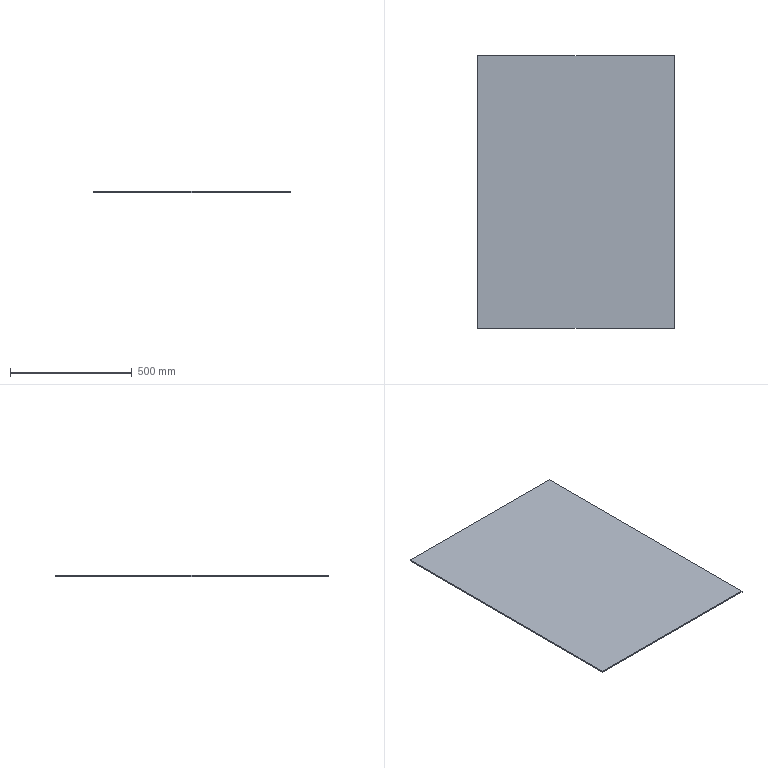Part | SolidWorks | features Extrusion 1 | 1 solid | 6 faces | box 807 x 1119 x 5 mm | volume 4515165 mm3 | plane 6
STEP:
#1=CARTESIAN_POINT('',(403.5,-559.5,0.));
#2=VERTEX_POINT('',#1);
#3=CARTESIAN_POINT('',(403.5,559.5,0.));
#4=VERTEX_POINT('',#3);
#5=CARTESIAN_POINT('',(403.5,559.5,0.));
#6=DIRECTION('',(0.,1.,0.));
#7=VECTOR('',#6,1000.);
#8=LINE('',#5,#7);
#9=EDGE_CURVE('',#2,#4,#8,.T.);
#10=ORIENTED_EDGE('',*,*,#9,.T.);
#11=CARTESIAN_POINT('',(403.5,559.5,5.));
#12=VERTEX_POINT('',#11);
#13=CARTESIAN_POINT('',(403.5,559.5,5.));
#14=DIRECTION('',(0.,0.,-1.));
#15=VECTOR('',#14,1000.);
#16=LINE('',#13,#15);
#17=EDGE_CURVE('',#12,#4,#16,.T.);
#18=ORIENTED_EDGE('',*,*,#17,.F.);
#19=CARTESIAN_POINT('',(403.5,-559.5,5.));
#20=VERTEX_POINT('',#19);
#21=CARTESIAN_POINT('',(403.5,559.5,5.));
#22=DIRECTION('',(0.,1.,0.));
#23=VECTOR('',#22,1000.);
#24=LINE('',#21,#23);
#25=EDGE_CURVE('',#20,#12,#24,.T.);
#26=ORIENTED_EDGE('',*,*,#25,.F.);
#27=CARTESIAN_POINT('',(403.5,-559.5,5.));
#28=DIRECTION('',(0.,0.,-1.));
#29=VECTOR('',#28,1000.);
#30=LINE('',#27,#29);
#31=EDGE_CURVE('',#20,#2,#30,.T.);
#32=ORIENTED_EDGE('',*,*,#31,.T.);
#33=EDGE_LOOP('',(#10,#18,#26,#32));
#34=FACE_OUTER_BOUND('',#33,.T.);
#35=CARTESIAN_POINT('',(403.5,559.5,5.));
#36=DIRECTION('',(-1.,0.,0.));
#37=DIRECTION('',(0.,-1.,0.));
#38=AXIS2_PLACEMENT_3D('',#35,#36,#37);
#39=PLANE('',#38);
#40=ADVANCED_FACE('',(#34),#39,.F.);
#41=CARTESIAN_POINT('',(-403.5,559.5,0.));
#42=VERTEX_POINT('',#41);
#43=CARTESIAN_POINT('',(-403.5,559.5,0.));
#44=DIRECTION('',(-1.,0.,0.));
#45=VECTOR('',#44,1000.);
#46=LINE('',#43,#45);
#47=EDGE_CURVE('',#4,#42,#46,.T.);
#48=ORIENTED_EDGE('',*,*,#47,.T.);
#49=CARTESIAN_POINT('',(-403.5,559.5,5.));
#50=VERTEX_POINT('',#49);
#51=CARTESIAN_POINT('',(-403.5,559.5,5.));
#52=DIRECTION('',(0.,0.,-1.));
#53=VECTOR('',#52,1000.);
#54=LINE('',#51,#53);
#55=EDGE_CURVE('',#50,#42,#54,.T.);
#56=ORIENTED_EDGE('',*,*,#55,.F.);
#57=CARTESIAN_POINT('',(-403.5,559.5,5.));
#58=DIRECTION('',(-1.,0.,0.));
#59=VECTOR('',#58,1000.);
#60=LINE('',#57,#59);
#61=EDGE_CURVE('',#12,#50,#60,.T.);
#62=ORIENTED_EDGE('',*,*,#61,.F.);
#63=ORIENTED_EDGE('',*,*,#17,.T.);
#64=EDGE_LOOP('',(#48,#56,#62,#63));
#65=FACE_OUTER_BOUND('',#64,.T.);
#66=CARTESIAN_POINT('',(-403.5,559.5,5.));
#67=DIRECTION('',(0.,-1.,0.));
#68=DIRECTION('',(0.,0.,-1.));
#69=AXIS2_PLACEMENT_3D('',#66,#67,#68);
#70=PLANE('',#69);
#71=ADVANCED_FACE('',(#65),#70,.F.);
#72=CARTESIAN_POINT('',(-403.5,-559.5,0.));
#73=VERTEX_POINT('',#72);
#74=CARTESIAN_POINT('',(-403.5,559.5,0.));
#75=DIRECTION('',(0.,-1.,0.));
#76=VECTOR('',#75,1000.);
#77=LINE('',#74,#76);
#78=EDGE_CURVE('',#42,#73,#77,.T.);
#79=ORIENTED_EDGE('',*,*,#78,.T.);
#80=CARTESIAN_POINT('',(-403.5,-559.5,5.));
#81=VERTEX_POINT('',#80);
#82=CARTESIAN_POINT('',(-403.5,-559.5,5.));
#83=DIRECTION('',(0.,0.,-1.));
#84=VECTOR('',#83,1000.);
#85=LINE('',#82,#84);
#86=EDGE_CURVE('',#81,#73,#85,.T.);
#87=ORIENTED_EDGE('',*,*,#86,.F.);
#88=CARTESIAN_POINT('',(-403.5,559.5,5.));
#89=DIRECTION('',(0.,-1.,0.));
#90=VECTOR('',#89,1000.);
#91=LINE('',#88,#90);
#92=EDGE_CURVE('',#50,#81,#91,.T.);
#93=ORIENTED_EDGE('',*,*,#92,.F.);
#94=ORIENTED_EDGE('',*,*,#55,.T.);
#95=EDGE_LOOP('',(#79,#87,#93,#94));
#96=FACE_OUTER_BOUND('',#95,.T.);
#97=CARTESIAN_POINT('',(-403.5,559.5,5.));
#98=DIRECTION('',(1.,0.,0.));
#99=DIRECTION('',(0.,1.,0.));
#100=AXIS2_PLACEMENT_3D('',#97,#98,#99);
#101=PLANE('',#100);
#102=ADVANCED_FACE('',(#96),#101,.F.);
#103=CARTESIAN_POINT('',(-403.5,-559.5,0.));
#104=DIRECTION('',(1.,0.,0.));
#105=VECTOR('',#104,1000.);
#106=LINE('',#103,#105);
#107=EDGE_CURVE('',#73,#2,#106,.T.);
#108=ORIENTED_EDGE('',*,*,#107,.T.);
#109=ORIENTED_EDGE('',*,*,#31,.F.);
#110=CARTESIAN_POINT('',(-403.5,-559.5,5.));
#111=DIRECTION('',(1.,0.,0.));
#112=VECTOR('',#111,1000.);
#113=LINE('',#110,#112);
#114=EDGE_CURVE('',#81,#20,#113,.T.);
#115=ORIENTED_EDGE('',*,*,#114,.F.);
#116=ORIENTED_EDGE('',*,*,#86,.T.);
#117=EDGE_LOOP('',(#108,#109,#115,#116));
#118=FACE_OUTER_BOUND('',#117,.T.);
#119=CARTESIAN_POINT('',(-403.5,-559.5,5.));
#120=DIRECTION('',(0.,1.,0.));
#121=DIRECTION('',(0.,0.,1.));
#122=AXIS2_PLACEMENT_3D('',#119,#120,#121);
#123=PLANE('',#122);
#124=ADVANCED_FACE('',(#118),#123,.F.);
#125=ORIENTED_EDGE('',*,*,#25,.T.);
#126=ORIENTED_EDGE('',*,*,#61,.T.);
#127=ORIENTED_EDGE('',*,*,#92,.T.);
#128=ORIENTED_EDGE('',*,*,#114,.T.);
#129=EDGE_LOOP('',(#125,#126,#127,#128));
#130=FACE_OUTER_BOUND('',#129,.T.);
#131=CARTESIAN_POINT('',(0.,0.,5.));
#132=DIRECTION('',(0.,0.,1.));
#133=DIRECTION('',(1.,0.,0.));
#134=AXIS2_PLACEMENT_3D('',#131,#132,#133);
#135=PLANE('',#134);
#136=ADVANCED_FACE('',(#130),#135,.T.);
#137=ORIENTED_EDGE('',*,*,#9,.F.);
#138=ORIENTED_EDGE('',*,*,#107,.F.);
#139=ORIENTED_EDGE('',*,*,#78,.F.);
#140=ORIENTED_EDGE('',*,*,#47,.F.);
#141=EDGE_LOOP('',(#137,#138,#139,#140));
#142=FACE_OUTER_BOUND('',#141,.T.);
#143=CARTESIAN_POINT('',(0.,0.,0.));
#144=DIRECTION('',(0.,0.,1.));
#145=DIRECTION('',(1.,0.,0.));
#146=AXIS2_PLACEMENT_3D('',#143,#144,#145);
#147=PLANE('',#146);
#148=ADVANCED_FACE('',(#142),#147,.F.);
#149=CLOSED_SHELL('',(#40,#71,#102,#124,#136,#148));
#150=MANIFOLD_SOLID_BREP('',#149);
#151=CARTESIAN_POINT('',(0.,0.,0.));
#152=DIRECTION('',(0.,0.,1.));
#153=DIRECTION('',(1.,0.,0.));
#154=AXIS2_PLACEMENT_3D('',#151,#152,#153);
#155=(LENGTH_UNIT()NAMED_UNIT(*)SI_UNIT(.MILLI.,.METRE.));
#156=UNCERTAINTY_MEASURE_WITH_UNIT(LENGTH_MEASURE(0.00001),#155,'','');
#157=(NAMED_UNIT(*)PLANE_ANGLE_UNIT()SI_UNIT($,.RADIAN.));
#158=(NAMED_UNIT(*)SI_UNIT($,.STERADIAN.)SOLID_ANGLE_UNIT());
#159=(GEOMETRIC_REPRESENTATION_CONTEXT(3)GLOBAL_UNCERTAINTY_ASSIGNED_CONTEXT((#156))GLOBAL_UNIT_ASSIGNED_CONTEXT((#155,#157,#158))REPRESENTATION_CONTEXT('',''));
#160=ADVANCED_BREP_SHAPE_REPRESENTATION('',(#150,#154),#159);